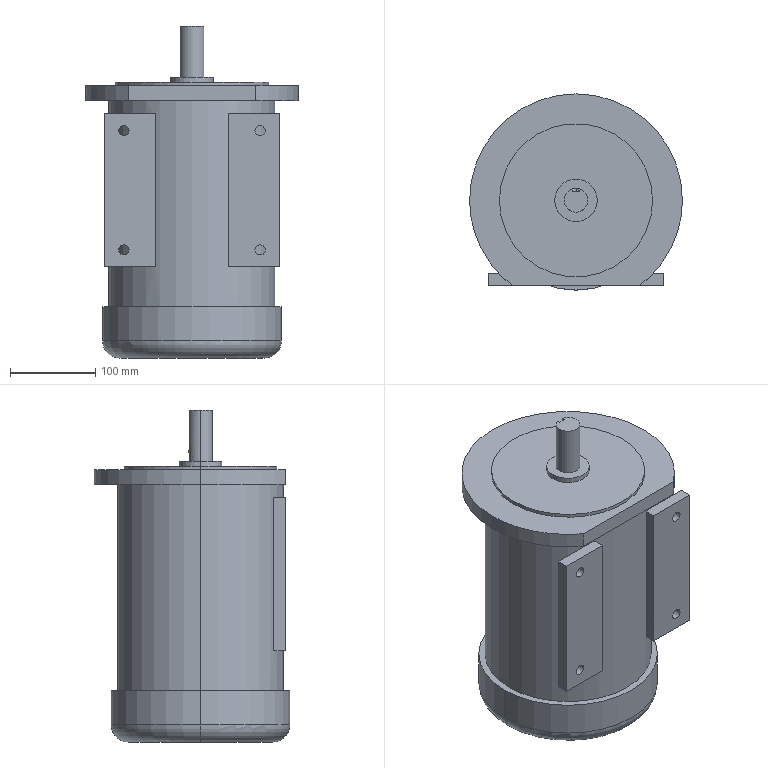Part | STEP file | Produce dryer line heating fan-MOYOT-Y100L2-4(3KW) | 1 solid | 48 faces | box 250 x 230 x 390 mm | volume 10532784 mm3 | cylinder 23 | plane 23 | torus 2 | commonest cylinder face diameters 12 x8 250 x3 8 x2 28 x2 50 x2 180 x2
STEP:
#1=CARTESIAN_POINT('',(74.,-100.,-193.));
#2=VERTEX_POINT('',#1);
#3=CARTESIAN_POINT('',(86.,-100.,-193.));
#4=VERTEX_POINT('',#3);
#5=CARTESIAN_POINT('',(80.,-100.,-193.));
#6=DIRECTION('',(0.,-1.,0.));
#7=DIRECTION('',(1.,0.,0.));
#8=AXIS2_PLACEMENT_3D('',#5,#6,#7);
#9=CIRCLE('',#8,6.);
#10=EDGE_CURVE('',#2,#4,#9,.T.);
#11=ORIENTED_EDGE('',*,*,#10,.T.);
#12=CARTESIAN_POINT('',(86.,-86.,-193.));
#13=VERTEX_POINT('',#12);
#14=CARTESIAN_POINT('',(86.,-100.,-193.));
#15=DIRECTION('',(0.,1.,0.));
#16=VECTOR('',#15,1000.);
#17=LINE('',#14,#16);
#18=EDGE_CURVE('',#4,#13,#17,.T.);
#19=ORIENTED_EDGE('',*,*,#18,.T.);
#20=CARTESIAN_POINT('',(74.,-86.,-193.));
#21=VERTEX_POINT('',#20);
#22=CARTESIAN_POINT('',(80.,-86.,-193.));
#23=DIRECTION('',(0.,-1.,0.));
#24=DIRECTION('',(1.,0.,0.));
#25=AXIS2_PLACEMENT_3D('',#22,#23,#24);
#26=CIRCLE('',#25,6.);
#27=EDGE_CURVE('',#21,#13,#26,.T.);
#28=ORIENTED_EDGE('',*,*,#27,.F.);
#29=CARTESIAN_POINT('',(74.,-100.,-193.));
#30=DIRECTION('',(0.,1.,0.));
#31=VECTOR('',#30,1000.);
#32=LINE('',#29,#31);
#33=EDGE_CURVE('',#2,#21,#32,.T.);
#34=ORIENTED_EDGE('',*,*,#33,.F.);
#35=EDGE_LOOP('',(#11,#19,#28,#34));
#36=FACE_OUTER_BOUND('',#35,.T.);
#37=CARTESIAN_POINT('',(80.,-100.,-193.));
#38=DIRECTION('',(0.,1.,0.));
#39=DIRECTION('',(-1.,0.,0.));
#40=AXIS2_PLACEMENT_3D('',#37,#38,#39);
#41=CYLINDRICAL_SURFACE('',#40,6.);
#42=ADVANCED_FACE('',(#36),#41,.F.);
#43=CARTESIAN_POINT('',(74.,-100.,-53.));
#44=VERTEX_POINT('',#43);
#45=CARTESIAN_POINT('',(86.,-100.,-53.));
#46=VERTEX_POINT('',#45);
#47=CARTESIAN_POINT('',(80.,-100.,-53.));
#48=DIRECTION('',(0.,-1.,0.));
#49=DIRECTION('',(1.,0.,0.));
#50=AXIS2_PLACEMENT_3D('',#47,#48,#49);
#51=CIRCLE('',#50,6.);
#52=EDGE_CURVE('',#44,#46,#51,.T.);
#53=ORIENTED_EDGE('',*,*,#52,.T.);
#54=CARTESIAN_POINT('',(86.,-86.,-53.));
#55=VERTEX_POINT('',#54);
#56=CARTESIAN_POINT('',(86.,-100.,-53.));
#57=DIRECTION('',(0.,1.,0.));
#58=VECTOR('',#57,1000.);
#59=LINE('',#56,#58);
#60=EDGE_CURVE('',#46,#55,#59,.T.);
#61=ORIENTED_EDGE('',*,*,#60,.T.);
#62=CARTESIAN_POINT('',(74.,-86.,-53.));
#63=VERTEX_POINT('',#62);
#64=CARTESIAN_POINT('',(80.,-86.,-53.));
#65=DIRECTION('',(0.,-1.,0.));
#66=DIRECTION('',(1.,0.,0.));
#67=AXIS2_PLACEMENT_3D('',#64,#65,#66);
#68=CIRCLE('',#67,6.);
#69=EDGE_CURVE('',#63,#55,#68,.T.);
#70=ORIENTED_EDGE('',*,*,#69,.F.);
#71=CARTESIAN_POINT('',(74.,-100.,-53.));
#72=DIRECTION('',(0.,1.,0.));
#73=VECTOR('',#72,1000.);
#74=LINE('',#71,#73);
#75=EDGE_CURVE('',#44,#63,#74,.T.);
#76=ORIENTED_EDGE('',*,*,#75,.F.);
#77=EDGE_LOOP('',(#53,#61,#70,#76));
#78=FACE_OUTER_BOUND('',#77,.T.);
#79=CARTESIAN_POINT('',(80.,-100.,-53.));
#80=DIRECTION('',(0.,1.,0.));
#81=DIRECTION('',(-1.,0.,0.));
#82=AXIS2_PLACEMENT_3D('',#79,#80,#81);
#83=CYLINDRICAL_SURFACE('',#82,6.);
#84=ADVANCED_FACE('',(#78),#83,.F.);
#85=CARTESIAN_POINT('',(-74.,-100.,-193.));
#86=VERTEX_POINT('',#85);
#87=CARTESIAN_POINT('',(-86.,-100.,-193.));
#88=VERTEX_POINT('',#87);
#89=CARTESIAN_POINT('',(-80.,-100.,-193.));
#90=DIRECTION('',(0.,1.,0.));
#91=DIRECTION('',(-1.,0.,0.));
#92=AXIS2_PLACEMENT_3D('',#89,#90,#91);
#93=CIRCLE('',#92,6.);
#94=EDGE_CURVE('',#86,#88,#93,.T.);
#95=ORIENTED_EDGE('',*,*,#94,.F.);
#96=CARTESIAN_POINT('',(-74.,-86.,-193.));
#97=VERTEX_POINT('',#96);
#98=CARTESIAN_POINT('',(-74.,-100.,-193.));
#99=DIRECTION('',(0.,1.,0.));
#100=VECTOR('',#99,1000.);
#101=LINE('',#98,#100);
#102=EDGE_CURVE('',#86,#97,#101,.T.);
#103=ORIENTED_EDGE('',*,*,#102,.T.);
#104=CARTESIAN_POINT('',(-86.,-86.,-193.));
#105=VERTEX_POINT('',#104);
#106=CARTESIAN_POINT('',(-80.,-86.,-193.));
#107=DIRECTION('',(0.,1.,0.));
#108=DIRECTION('',(-1.,0.,0.));
#109=AXIS2_PLACEMENT_3D('',#106,#107,#108);
#110=CIRCLE('',#109,6.);
#111=EDGE_CURVE('',#97,#105,#110,.T.);
#112=ORIENTED_EDGE('',*,*,#111,.T.);
#113=CARTESIAN_POINT('',(-86.,-100.,-193.));
#114=DIRECTION('',(0.,1.,0.));
#115=VECTOR('',#114,1000.);
#116=LINE('',#113,#115);
#117=EDGE_CURVE('',#88,#105,#116,.T.);
#118=ORIENTED_EDGE('',*,*,#117,.F.);
#119=EDGE_LOOP('',(#95,#103,#112,#118));
#120=FACE_OUTER_BOUND('',#119,.T.);
#121=CARTESIAN_POINT('',(-80.,-100.,-193.));
#122=DIRECTION('',(0.,1.,0.));
#123=DIRECTION('',(-1.,0.,0.));
#124=AXIS2_PLACEMENT_3D('',#121,#122,#123);
#125=CYLINDRICAL_SURFACE('',#124,6.);
#126=ADVANCED_FACE('',(#120),#125,.F.);
#127=CARTESIAN_POINT('',(-74.,-100.,-53.));
#128=VERTEX_POINT('',#127);
#129=CARTESIAN_POINT('',(-86.,-100.,-53.));
#130=VERTEX_POINT('',#129);
#131=CARTESIAN_POINT('',(-80.,-100.,-53.));
#132=DIRECTION('',(0.,1.,0.));
#133=DIRECTION('',(-1.,0.,0.));
#134=AXIS2_PLACEMENT_3D('',#131,#132,#133);
#135=CIRCLE('',#134,6.);
#136=EDGE_CURVE('',#128,#130,#135,.T.);
#137=ORIENTED_EDGE('',*,*,#136,.F.);
#138=CARTESIAN_POINT('',(-74.,-86.,-53.));
#139=VERTEX_POINT('',#138);
#140=CARTESIAN_POINT('',(-74.,-100.,-53.));
#141=DIRECTION('',(0.,1.,0.));
#142=VECTOR('',#141,1000.);
#143=LINE('',#140,#142);
#144=EDGE_CURVE('',#128,#139,#143,.T.);
#145=ORIENTED_EDGE('',*,*,#144,.T.);
#146=CARTESIAN_POINT('',(-86.,-86.,-53.));
#147=VERTEX_POINT('',#146);
#148=CARTESIAN_POINT('',(-80.,-86.,-53.));
#149=DIRECTION('',(0.,1.,0.));
#150=DIRECTION('',(-1.,0.,0.));
#151=AXIS2_PLACEMENT_3D('',#148,#149,#150);
#152=CIRCLE('',#151,6.);
#153=EDGE_CURVE('',#139,#147,#152,.T.);
#154=ORIENTED_EDGE('',*,*,#153,.T.);
#155=CARTESIAN_POINT('',(-86.,-100.,-53.));
#156=DIRECTION('',(0.,1.,0.));
#157=VECTOR('',#156,1000.);
#158=LINE('',#155,#157);
#159=EDGE_CURVE('',#130,#147,#158,.T.);
#160=ORIENTED_EDGE('',*,*,#159,.F.);
#161=EDGE_LOOP('',(#137,#145,#154,#160));
#162=FACE_OUTER_BOUND('',#161,.T.);
#163=CARTESIAN_POINT('',(-80.,-100.,-53.));
#164=DIRECTION('',(0.,1.,0.));
#165=DIRECTION('',(-1.,0.,0.));
#166=AXIS2_PLACEMENT_3D('',#163,#164,#165);
#167=CYLINDRICAL_SURFACE('',#166,6.);
#168=ADVANCED_FACE('',(#162),#167,.F.);
#169=CARTESIAN_POINT('',(105.,0.,-300.));
#170=VERTEX_POINT('',#169);
#171=CARTESIAN_POINT('',(-105.,0.,-300.));
#172=VERTEX_POINT('',#171);
#173=CARTESIAN_POINT('',(0.,0.,-300.));
#174=DIRECTION('',(0.,0.,1.));
#175=DIRECTION('',(-1.,0.,0.));
#176=AXIS2_PLACEMENT_3D('',#173,#174,#175);
#177=CIRCLE('',#176,105.);
#178=EDGE_CURVE('',#170,#172,#177,.T.);
#179=ORIENTED_EDGE('',*,*,#178,.F.);
#180=CARTESIAN_POINT('',(85.,0.,-320.));
#181=VERTEX_POINT('',#180);
#182=CARTESIAN_POINT('',(85.,0.,-300.));
#183=DIRECTION('',(0.,1.,0.));
#184=DIRECTION('',(-1.,0.,0.));
#185=AXIS2_PLACEMENT_3D('',#182,#183,#184);
#186=CIRCLE('',#185,20.);
#187=EDGE_CURVE('',#170,#181,#186,.T.);
#188=ORIENTED_EDGE('',*,*,#187,.T.);
#189=CARTESIAN_POINT('',(-85.,0.,-320.));
#190=VERTEX_POINT('',#189);
#191=CARTESIAN_POINT('',(0.,0.,-320.));
#192=DIRECTION('',(0.,0.,-1.));
#193=DIRECTION('',(-1.,0.,0.));
#194=AXIS2_PLACEMENT_3D('',#191,#192,#193);
#195=CIRCLE('',#194,85.);
#196=EDGE_CURVE('',#190,#181,#195,.T.);
#197=ORIENTED_EDGE('',*,*,#196,.F.);
#198=CARTESIAN_POINT('',(-85.,0.,-300.));
#199=DIRECTION('',(0.,-1.,0.));
#200=DIRECTION('',(0.,0.,-1.));
#201=AXIS2_PLACEMENT_3D('',#198,#199,#200);
#202=CIRCLE('',#201,20.);
#203=EDGE_CURVE('',#172,#190,#202,.T.);
#204=ORIENTED_EDGE('',*,*,#203,.F.);
#205=EDGE_LOOP('',(#179,#188,#197,#204));
#206=FACE_OUTER_BOUND('',#205,.T.);
#207=CARTESIAN_POINT('',(0.,0.,-300.));
#208=DIRECTION('',(0.,0.,-1.));
#209=DIRECTION('',(-1.,0.,0.));
#210=AXIS2_PLACEMENT_3D('',#207,#208,#209);
#211=TOROIDAL_SURFACE('',#210,85.,20.);
#212=ADVANCED_FACE('',(#206),#211,.T.);
#213=ORIENTED_EDGE('',*,*,#178,.T.);
#214=CARTESIAN_POINT('',(-105.,0.,-260.));
#215=VERTEX_POINT('',#214);
#216=CARTESIAN_POINT('',(-105.,0.,-320.));
#217=DIRECTION('',(0.,0.,1.));
#218=VECTOR('',#217,1000.);
#219=LINE('',#216,#218);
#220=EDGE_CURVE('',#172,#215,#219,.T.);
#221=ORIENTED_EDGE('',*,*,#220,.T.);
#222=CARTESIAN_POINT('',(105.,0.,-260.));
#223=VERTEX_POINT('',#222);
#224=CARTESIAN_POINT('',(0.,0.,-260.));
#225=DIRECTION('',(0.,0.,-1.));
#226=DIRECTION('',(-1.,0.,0.));
#227=AXIS2_PLACEMENT_3D('',#224,#225,#226);
#228=CIRCLE('',#227,105.);
#229=EDGE_CURVE('',#215,#223,#228,.T.);
#230=ORIENTED_EDGE('',*,*,#229,.T.);
#231=CARTESIAN_POINT('',(105.,0.,-320.));
#232=DIRECTION('',(0.,0.,1.));
#233=VECTOR('',#232,1000.);
#234=LINE('',#231,#233);
#235=EDGE_CURVE('',#170,#223,#234,.T.);
#236=ORIENTED_EDGE('',*,*,#235,.F.);
#237=EDGE_LOOP('',(#213,#221,#230,#236));
#238=FACE_OUTER_BOUND('',#237,.T.);
#239=CARTESIAN_POINT('',(0.,0.,-320.));
#240=DIRECTION('',(0.,0.,1.));
#241=DIRECTION('',(1.,0.,0.));
#242=AXIS2_PLACEMENT_3D('',#239,#240,#241);
#243=CYLINDRICAL_SURFACE('',#242,105.);
#244=ADVANCED_FACE('',(#238),#243,.T.);
#245=CARTESIAN_POINT('',(-97.5,0.,-260.));
#246=VERTEX_POINT('',#245);
#247=CARTESIAN_POINT('',(97.5,0.,-260.));
#248=VERTEX_POINT('',#247);
#249=CARTESIAN_POINT('',(0.,0.,-260.));
#250=DIRECTION('',(0.,0.,-1.));
#251=DIRECTION('',(-1.,0.,0.));
#252=AXIS2_PLACEMENT_3D('',#249,#250,#251);
#253=CIRCLE('',#252,97.5);
#254=EDGE_CURVE('',#246,#248,#253,.T.);
#255=ORIENTED_EDGE('',*,*,#254,.F.);
#256=CARTESIAN_POINT('',(-97.5,0.,-18.));
#257=VERTEX_POINT('',#256);
#258=CARTESIAN_POINT('',(-97.5,0.,-260.));
#259=DIRECTION('',(0.,0.,1.));
#260=VECTOR('',#259,1000.);
#261=LINE('',#258,#260);
#262=EDGE_CURVE('',#246,#257,#261,.T.);
#263=ORIENTED_EDGE('',*,*,#262,.T.);
#264=CARTESIAN_POINT('',(97.5,0.,-18.));
#265=VERTEX_POINT('',#264);
#266=CARTESIAN_POINT('',(0.,0.,-18.));
#267=DIRECTION('',(0.,0.,-1.));
#268=DIRECTION('',(1.,0.,0.));
#269=AXIS2_PLACEMENT_3D('',#266,#267,#268);
#270=CIRCLE('',#269,97.5);
#271=EDGE_CURVE('',#257,#265,#270,.T.);
#272=ORIENTED_EDGE('',*,*,#271,.T.);
#273=CARTESIAN_POINT('',(97.5,0.,-260.));
#274=DIRECTION('',(0.,0.,1.));
#275=VECTOR('',#274,1000.);
#276=LINE('',#273,#275);
#277=EDGE_CURVE('',#248,#265,#276,.T.);
#278=ORIENTED_EDGE('',*,*,#277,.F.);
#279=EDGE_LOOP('',(#255,#263,#272,#278));
#280=FACE_OUTER_BOUND('',#279,.T.);
#281=CARTESIAN_POINT('',(0.,0.,-260.));
#282=DIRECTION('',(0.,0.,1.));
#283=DIRECTION('',(1.,0.,0.));
#284=AXIS2_PLACEMENT_3D('',#281,#282,#283);
#285=CYLINDRICAL_SURFACE('',#284,97.5);
#286=ADVANCED_FACE('',(#280),#285,.T.);
#287=CARTESIAN_POINT('',(14.,0.,70.));
#288=VERTEX_POINT('',#287);
#289=CARTESIAN_POINT('',(4.,13.416,70.));
#290=VERTEX_POINT('',#289);
#291=CARTESIAN_POINT('',(0.,0.,70.));
#292=DIRECTION('',(0.,0.,1.));
#293=DIRECTION('',(1.,0.,0.));
#294=AXIS2_PLACEMENT_3D('',#291,#292,#293);
#295=CIRCLE('',#294,14.);
#296=EDGE_CURVE('',#288,#290,#295,.T.);
#297=ORIENTED_EDGE('',*,*,#296,.F.);
#298=CARTESIAN_POINT('',(14.,0.,10.));
#299=VERTEX_POINT('',#298);
#300=CARTESIAN_POINT('',(14.,0.,70.));
#301=DIRECTION('',(0.,0.,-1.));
#302=VECTOR('',#301,1000.);
#303=LINE('',#300,#302);
#304=EDGE_CURVE('',#288,#299,#303,.T.);
#305=ORIENTED_EDGE('',*,*,#304,.T.);
#306=CARTESIAN_POINT('',(-14.,0.,10.));
#307=VERTEX_POINT('',#306);
#308=CARTESIAN_POINT('',(0.,0.,10.));
#309=DIRECTION('',(0.,0.,1.));
#310=DIRECTION('',(1.,0.,0.));
#311=AXIS2_PLACEMENT_3D('',#308,#309,#310);
#312=CIRCLE('',#311,14.);
#313=EDGE_CURVE('',#299,#307,#312,.T.);
#314=ORIENTED_EDGE('',*,*,#313,.T.);
#315=CARTESIAN_POINT('',(-14.,0.,70.));
#316=VERTEX_POINT('',#315);
#317=CARTESIAN_POINT('',(-14.,0.,70.));
#318=DIRECTION('',(0.,0.,-1.));
#319=VECTOR('',#318,1000.);
#320=LINE('',#317,#319);
#321=EDGE_CURVE('',#316,#307,#320,.T.);
#322=ORIENTED_EDGE('',*,*,#321,.F.);
#323=CARTESIAN_POINT('',(-4.,13.416,70.));
#324=VERTEX_POINT('',#323);
#325=CARTESIAN_POINT('',(0.,0.,70.));
#326=DIRECTION('',(0.,0.,1.));
#327=DIRECTION('',(1.,0.,0.));
#328=AXIS2_PLACEMENT_3D('',#325,#326,#327);
#329=CIRCLE('',#328,14.);
#330=EDGE_CURVE('',#324,#316,#329,.T.);
#331=ORIENTED_EDGE('',*,*,#330,.F.);
#332=CARTESIAN_POINT('',(-4.,13.416,24.));
#333=VERTEX_POINT('',#332);
#334=CARTESIAN_POINT('',(-4.,13.416,70.));
#335=DIRECTION('',(0.,0.,-1.));
#336=VECTOR('',#335,1000.);
#337=LINE('',#334,#336);
#338=EDGE_CURVE('',#324,#333,#337,.T.);
#339=ORIENTED_EDGE('',*,*,#338,.T.);
#340=CARTESIAN_POINT('',(0.,14.,20.));
#341=VERTEX_POINT('',#340);
#342=CARTESIAN_POINT('',(-4.,13.416,24.));
#343=CARTESIAN_POINT('',(-4.,13.416,23.734));
#344=CARTESIAN_POINT('',(-3.974,13.424,23.474));
#345=CARTESIAN_POINT('',(-3.871,13.454,22.961));
#346=CARTESIAN_POINT('',(-3.794,13.477,22.706));
#347=CARTESIAN_POINT('',(-3.593,13.531,22.223));
#348=CARTESIAN_POINT('',(-3.47,13.564,21.994));
#349=CARTESIAN_POINT('',(-3.18,13.635,21.56));
#350=CARTESIAN_POINT('',(-3.013,13.673,21.356));
#351=CARTESIAN_POINT('',(-2.646,13.749,20.989));
#352=CARTESIAN_POINT('',(-2.446,13.786,20.824));
#353=CARTESIAN_POINT('',(-2.009,13.857,20.531));
#354=CARTESIAN_POINT('',(-1.779,13.889,20.408));
#355=CARTESIAN_POINT('',(-1.299,13.942,20.208));
#356=CARTESIAN_POINT('',(-1.046,13.963,20.13));
#357=CARTESIAN_POINT('',(-0.5278,13.992,20.026));
#358=CARTESIAN_POINT('',(-0.2656,14.,20.));
#359=CARTESIAN_POINT('',(0.,14.,20.));
#360=B_SPLINE_CURVE_WITH_KNOTS('',3,(#342,#343,#344,#345,#346,#347,#348,#349,#350,#351,#352,#353,#354,#355,#356,#357,#358,#359),.UNSPECIFIED.,.F.,.F.,(4,2,2,2,2,2,2,2,4),(0.,0.0007852,0.00157,0.002356,0.003141,0.003926,0.004711,0.005496,0.006282),.UNSPECIFIED.);
#361=EDGE_CURVE('',#333,#341,#360,.T.);
#362=ORIENTED_EDGE('',*,*,#361,.T.);
#363=CARTESIAN_POINT('',(4.,13.416,24.));
#364=VERTEX_POINT('',#363);
#365=CARTESIAN_POINT('',(0.,14.,20.));
#366=CARTESIAN_POINT('',(0.2656,14.,20.));
#367=CARTESIAN_POINT('',(0.5265,13.992,20.026));
#368=CARTESIAN_POINT('',(1.039,13.964,20.129));
#369=CARTESIAN_POINT('',(1.294,13.942,20.206));
#370=CARTESIAN_POINT('',(1.778,13.889,20.407));
#371=CARTESIAN_POINT('',(2.007,13.857,20.53));
#372=CARTESIAN_POINT('',(2.44,13.787,20.82));
#373=CARTESIAN_POINT('',(2.645,13.749,20.988));
#374=CARTESIAN_POINT('',(3.011,13.674,21.354));
#375=CARTESIAN_POINT('',(3.176,13.636,21.555));
#376=CARTESIAN_POINT('',(3.469,13.564,21.991));
#377=CARTESIAN_POINT('',(3.592,13.532,22.221));
#378=CARTESIAN_POINT('',(3.792,13.477,22.702));
#379=CARTESIAN_POINT('',(3.87,13.455,22.954));
#380=CARTESIAN_POINT('',(3.974,13.424,23.472));
#381=CARTESIAN_POINT('',(4.,13.416,23.734));
#382=CARTESIAN_POINT('',(4.,13.416,24.));
#383=B_SPLINE_CURVE_WITH_KNOTS('',3,(#365,#366,#367,#368,#369,#370,#371,#372,#373,#374,#375,#376,#377,#378,#379,#380,#381,#382),.UNSPECIFIED.,.F.,.F.,(4,2,2,2,2,2,2,2,4),(0.,0.0007852,0.00157,0.002356,0.003141,0.003926,0.004711,0.005496,0.006282),.UNSPECIFIED.);
#384=EDGE_CURVE('',#341,#364,#383,.T.);
#385=ORIENTED_EDGE('',*,*,#384,.T.);
#386=CARTESIAN_POINT('',(4.,13.416,70.));
#387=DIRECTION('',(0.,0.,1.));
#388=VECTOR('',#387,1000.);
#389=LINE('',#386,#388);
#390=EDGE_CURVE('',#364,#290,#389,.T.);
#391=ORIENTED_EDGE('',*,*,#390,.T.);
#392=EDGE_LOOP('',(#297,#305,#314,#322,#331,#339,#362,#385,#391));
#393=FACE_OUTER_BOUND('',#392,.T.);
#394=CARTESIAN_POINT('',(0.,0.,70.));
#395=DIRECTION('',(0.,0.,-1.));
#396=DIRECTION('',(-1.,0.,0.));
#397=AXIS2_PLACEMENT_3D('',#394,#395,#396);
#398=CYLINDRICAL_SURFACE('',#397,14.);
#399=ADVANCED_FACE('',(#393),#398,.T.);
#400=CARTESIAN_POINT('',(25.,0.,10.));
#401=VERTEX_POINT('',#400);
#402=CARTESIAN_POINT('',(-25.,0.,10.));
#403=VERTEX_POINT('',#402);
#404=CARTESIAN_POINT('',(0.,0.,10.));
#405=DIRECTION('',(0.,0.,1.));
#406=DIRECTION('',(1.,0.,0.));
#407=AXIS2_PLACEMENT_3D('',#404,#405,#406);
#408=CIRCLE('',#407,25.);
#409=EDGE_CURVE('',#401,#403,#408,.T.);
#410=ORIENTED_EDGE('',*,*,#409,.F.);
#411=CARTESIAN_POINT('',(25.,0.,4.));
#412=VERTEX_POINT('',#411);
#413=CARTESIAN_POINT('',(25.,0.,10.));
#414=DIRECTION('',(0.,0.,-1.));
#415=VECTOR('',#414,1000.);
#416=LINE('',#413,#415);
#417=EDGE_CURVE('',#401,#412,#416,.T.);
#418=ORIENTED_EDGE('',*,*,#417,.T.);
#419=CARTESIAN_POINT('',(-25.,0.,4.));
#420=VERTEX_POINT('',#419);
#421=CARTESIAN_POINT('',(0.,0.,4.));
#422=DIRECTION('',(0.,0.,1.));
#423=DIRECTION('',(1.,0.,0.));
#424=AXIS2_PLACEMENT_3D('',#421,#422,#423);
#425=CIRCLE('',#424,25.);
#426=EDGE_CURVE('',#412,#420,#425,.T.);
#427=ORIENTED_EDGE('',*,*,#426,.T.);
#428=CARTESIAN_POINT('',(-25.,0.,10.));
#429=DIRECTION('',(0.,0.,-1.));
#430=VECTOR('',#429,1000.);
#431=LINE('',#428,#430);
#432=EDGE_CURVE('',#403,#420,#431,.T.);
#433=ORIENTED_EDGE('',*,*,#432,.F.);
#434=EDGE_LOOP('',(#410,#418,#427,#433));
#435=FACE_OUTER_BOUND('',#434,.T.);
#436=CARTESIAN_POINT('',(0.,0.,10.));
#437=DIRECTION('',(0.,0.,-1.));
#438=DIRECTION('',(-1.,0.,0.));
#439=AXIS2_PLACEMENT_3D('',#436,#437,#438);
#440=CYLINDRICAL_SURFACE('',#439,25.);
#441=ADVANCED_FACE('',(#435),#440,.T.);
#442=CARTESIAN_POINT('',(90.,0.,4.));
#443=VERTEX_POINT('',#442);
#444=CARTESIAN_POINT('',(-90.,0.,4.));
#445=VERTEX_POINT('',#444);
#446=CARTESIAN_POINT('',(0.,0.,4.));
#447=DIRECTION('',(0.,0.,1.));
#448=DIRECTION('',(1.,0.,0.));
#449=AXIS2_PLACEMENT_3D('',#446,#447,#448);
#450=CIRCLE('',#449,90.);
#451=EDGE_CURVE('',#443,#445,#450,.T.);
#452=ORIENTED_EDGE('',*,*,#451,.F.);
#453=CARTESIAN_POINT('',(90.,0.,0.));
#454=VERTEX_POINT('',#453);
#455=CARTESIAN_POINT('',(90.,0.,4.));
#456=DIRECTION('',(0.,0.,-1.));
#457=VECTOR('',#456,1000.);
#458=LINE('',#455,#457);
#459=EDGE_CURVE('',#443,#454,#458,.T.);
#460=ORIENTED_EDGE('',*,*,#459,.T.);
#461=CARTESIAN_POINT('',(-90.,0.,0.));
#462=VERTEX_POINT('',#461);
#463=CARTESIAN_POINT('',(0.,0.,0.));
#464=DIRECTION('',(0.,0.,1.));
#465=DIRECTION('',(1.,0.,0.));
#466=AXIS2_PLACEMENT_3D('',#463,#464,#465);
#467=CIRCLE('',#466,90.);
#468=EDGE_CURVE('',#454,#462,#467,.T.);
#469=ORIENTED_EDGE('',*,*,#468,.T.);
#470=CARTESIAN_POINT('',(-90.,0.,4.));
#471=DIRECTION('',(0.,0.,-1.));
#472=VECTOR('',#471,1000.);
#473=LINE('',#470,#472);
#474=EDGE_CURVE('',#445,#462,#473,.T.);
#475=ORIENTED_EDGE('',*,*,#474,.F.);
#476=EDGE_LOOP('',(#452,#460,#469,#475));
#477=FACE_OUTER_BOUND('',#476,.T.);
#478=CARTESIAN_POINT('',(0.,0.,4.));
#479=DIRECTION('',(0.,0.,-1.));
#480=DIRECTION('',(-1.,0.,0.));
#481=AXIS2_PLACEMENT_3D('',#478,#479,#480);
#482=CYLINDRICAL_SURFACE('',#481,90.);
#483=ADVANCED_FACE('',(#477),#482,.T.);
#484=CARTESIAN_POINT('',(125.,0.,-18.));
#485=VERTEX_POINT('',#484);
#486=CARTESIAN_POINT('',(-125.,0.,-18.));
#487=VERTEX_POINT('',#486);
#488=CARTESIAN_POINT('',(0.,0.,-18.));
#489=DIRECTION('',(0.,0.,1.));
#490=DIRECTION('',(1.,0.,0.));
#491=AXIS2_PLACEMENT_3D('',#488,#489,#490);
#492=CIRCLE('',#491,125.);
#493=EDGE_CURVE('',#485,#487,#492,.T.);
#494=ORIENTED_EDGE('',*,*,#493,.T.);
#495=CARTESIAN_POINT('',(-125.,0.,0.));
#496=VERTEX_POINT('',#495);
#497=CARTESIAN_POINT('',(-125.,0.,-18.));
#498=DIRECTION('',(0.,0.,1.));
#499=VECTOR('',#498,1000.);
#500=LINE('',#497,#499);
#501=EDGE_CURVE('',#487,#496,#500,.T.);
#502=ORIENTED_EDGE('',*,*,#501,.T.);
#503=CARTESIAN_POINT('',(125.,0.,0.));
#504=VERTEX_POINT('',#503);
#505=CARTESIAN_POINT('',(0.,0.,0.));
#506=DIRECTION('',(0.,0.,1.));
#507=DIRECTION('',(1.,0.,0.));
#508=AXIS2_PLACEMENT_3D('',#505,#506,#507);
#509=CIRCLE('',#508,125.);
#510=EDGE_CURVE('',#504,#496,#509,.T.);
#511=ORIENTED_EDGE('',*,*,#510,.F.);
#512=CARTESIAN_POINT('',(125.,0.,-18.));
#513=DIRECTION('',(0.,0.,1.));
#514=VECTOR('',#513,1000.);
#515=LINE('',#512,#514);
#516=EDGE_CURVE('',#485,#504,#515,.T.);
#517=ORIENTED_EDGE('',*,*,#516,.F.);
#518=EDGE_LOOP('',(#494,#502,#511,#517));
#519=FACE_OUTER_BOUND('',#518,.T.);
#520=CARTESIAN_POINT('',(0.,0.,-18.));
#521=DIRECTION('',(0.,0.,1.));
#522=DIRECTION('',(1.,0.,0.));
#523=AXIS2_PLACEMENT_3D('',#520,#521,#522);
#524=CYLINDRICAL_SURFACE('',#523,125.);
#525=ADVANCED_FACE('',(#519),#524,.T.);
#526=CARTESIAN_POINT('',(75.,-100.,-18.));
#527=VERTEX_POINT('',#526);
#528=CARTESIAN_POINT('',(0.,0.,-18.));
#529=DIRECTION('',(0.,0.,1.));
#530=DIRECTION('',(1.,0.,0.));
#531=AXIS2_PLACEMENT_3D('',#528,#529,#530);
#532=CIRCLE('',#531,125.);
#533=EDGE_CURVE('',#527,#485,#532,.T.);
#534=ORIENTED_EDGE('',*,*,#533,.T.);
#535=ORIENTED_EDGE('',*,*,#516,.T.);
#536=CARTESIAN_POINT('',(75.,-100.,0.));
#537=VERTEX_POINT('',#536);
#538=CARTESIAN_POINT('',(0.,0.,0.));
#539=DIRECTION('',(0.,0.,1.));
#540=DIRECTION('',(1.,0.,0.));
#541=AXIS2_PLACEMENT_3D('',#538,#539,#540);
#542=CIRCLE('',#541,125.);
#543=EDGE_CURVE('',#537,#504,#542,.T.);
#544=ORIENTED_EDGE('',*,*,#543,.F.);
#545=CARTESIAN_POINT('',(75.,-100.,-18.));
#546=DIRECTION('',(0.,0.,1.));
#547=VECTOR('',#546,1000.);
#548=LINE('',#545,#547);
#549=EDGE_CURVE('',#527,#537,#548,.T.);
#550=ORIENTED_EDGE('',*,*,#549,.F.);
#551=EDGE_LOOP('',(#534,#535,#544,#550));
#552=FACE_OUTER_BOUND('',#551,.T.);
#553=CARTESIAN_POINT('',(0.,0.,-18.));
#554=DIRECTION('',(0.,0.,1.));
#555=DIRECTION('',(1.,0.,0.));
#556=AXIS2_PLACEMENT_3D('',#553,#554,#555);
#557=CYLINDRICAL_SURFACE('',#556,125.);
#558=ADVANCED_FACE('',(#552),#557,.T.);
#559=ORIENTED_EDGE('',*,*,#69,.T.);
#560=CARTESIAN_POINT('',(80.,-86.,-53.));
#561=DIRECTION('',(0.,-1.,0.));
#562=DIRECTION('',(1.,0.,0.));
#563=AXIS2_PLACEMENT_3D('',#560,#561,#562);
#564=CIRCLE('',#563,6.);
#565=EDGE_CURVE('',#55,#63,#564,.T.);
#566=ORIENTED_EDGE('',*,*,#565,.T.);
#567=EDGE_LOOP('',(#559,#566));
#568=FACE_BOUND('',#567,.T.);
#569=CARTESIAN_POINT('',(45.937,-86.,-213.));
#570=VERTEX_POINT('',#569);
#571=CARTESIAN_POINT('',(102.5,-86.,-213.));
#572=VERTEX_POINT('',#571);
#573=CARTESIAN_POINT('',(102.5,-86.,-213.));
#574=DIRECTION('',(1.,0.,0.));
#575=VECTOR('',#574,1000.);
#576=LINE('',#573,#575);
#577=EDGE_CURVE('',#570,#572,#576,.T.);
#578=ORIENTED_EDGE('',*,*,#577,.F.);
#579=CARTESIAN_POINT('',(45.937,-86.,-33.));
#580=VERTEX_POINT('',#579);
#581=CARTESIAN_POINT('',(45.937,-86.,-260.));
#582=DIRECTION('',(0.,0.,1.));
#583=VECTOR('',#582,1000.);
#584=LINE('',#581,#583);
#585=EDGE_CURVE('',#570,#580,#584,.T.);
#586=ORIENTED_EDGE('',*,*,#585,.T.);
#587=CARTESIAN_POINT('',(102.5,-86.,-33.));
#588=VERTEX_POINT('',#587);
#589=CARTESIAN_POINT('',(102.5,-86.,-33.));
#590=DIRECTION('',(1.,0.,0.));
#591=VECTOR('',#590,1000.);
#592=LINE('',#589,#591);
#593=EDGE_CURVE('',#580,#588,#592,.T.);
#594=ORIENTED_EDGE('',*,*,#593,.T.);
#595=CARTESIAN_POINT('',(102.5,-86.,-213.));
#596=DIRECTION('',(0.,0.,1.));
#597=VECTOR('',#596,1000.);
#598=LINE('',#595,#597);
#599=EDGE_CURVE('',#572,#588,#598,.T.);
#600=ORIENTED_EDGE('',*,*,#599,.F.);
#601=EDGE_LOOP('',(#578,#586,#594,#600));
#602=FACE_OUTER_BOUND('',#601,.T.);
#603=ORIENTED_EDGE('',*,*,#27,.T.);
#604=CARTESIAN_POINT('',(80.,-86.,-193.));
#605=DIRECTION('',(0.,-1.,0.));
#606=DIRECTION('',(1.,0.,0.));
#607=AXIS2_PLACEMENT_3D('',#604,#605,#606);
#608=CIRCLE('',#607,6.);
#609=EDGE_CURVE('',#13,#21,#608,.T.);
#610=ORIENTED_EDGE('',*,*,#609,.T.);
#611=EDGE_LOOP('',(#603,#610));
#612=FACE_BOUND('',#611,.T.);
#613=CARTESIAN_POINT('',(102.5,-86.,-213.));
#614=DIRECTION('',(0.,-1.,0.));
#615=DIRECTION('',(0.,0.,-1.));
#616=AXIS2_PLACEMENT_3D('',#613,#614,#615);
#617=PLANE('',#616);
#618=ADVANCED_FACE('',(#568,#602,#612),#617,.F.);
#619=ORIENTED_EDGE('',*,*,#52,.F.);
#620=CARTESIAN_POINT('',(80.,-100.,-53.));
#621=DIRECTION('',(0.,-1.,0.));
#622=DIRECTION('',(1.,0.,0.));
#623=AXIS2_PLACEMENT_3D('',#620,#621,#622);
#624=CIRCLE('',#623,6.);
#625=EDGE_CURVE('',#46,#44,#624,.T.);
#626=ORIENTED_EDGE('',*,*,#625,.F.);
#627=EDGE_LOOP('',(#619,#626));
#628=FACE_BOUND('',#627,.T.);
#629=CARTESIAN_POINT('',(102.5,-100.,-33.));
#630=VERTEX_POINT('',#629);
#631=CARTESIAN_POINT('',(42.5,-100.,-33.));
#632=VERTEX_POINT('',#631);
#633=CARTESIAN_POINT('',(42.5,-100.,-33.));
#634=DIRECTION('',(-1.,0.,0.));
#635=VECTOR('',#634,1000.);
#636=LINE('',#633,#635);
#637=EDGE_CURVE('',#630,#632,#636,.T.);
#638=ORIENTED_EDGE('',*,*,#637,.T.);
#639=CARTESIAN_POINT('',(42.5,-100.,-213.));
#640=VERTEX_POINT('',#639);
#641=CARTESIAN_POINT('',(42.5,-100.,-213.));
#642=DIRECTION('',(0.,0.,1.));
#643=VECTOR('',#642,1000.);
#644=LINE('',#641,#643);
#645=EDGE_CURVE('',#640,#632,#644,.T.);
#646=ORIENTED_EDGE('',*,*,#645,.F.);
#647=CARTESIAN_POINT('',(102.5,-100.,-213.));
#648=VERTEX_POINT('',#647);
#649=CARTESIAN_POINT('',(42.5,-100.,-213.));
#650=DIRECTION('',(-1.,0.,0.));
#651=VECTOR('',#650,1000.);
#652=LINE('',#649,#651);
#653=EDGE_CURVE('',#648,#640,#652,.T.);
#654=ORIENTED_EDGE('',*,*,#653,.F.);
#655=CARTESIAN_POINT('',(102.5,-100.,-213.));
#656=DIRECTION('',(0.,0.,1.));
#657=VECTOR('',#656,1000.);
#658=LINE('',#655,#657);
#659=EDGE_CURVE('',#648,#630,#658,.T.);
#660=ORIENTED_EDGE('',*,*,#659,.T.);
#661=EDGE_LOOP('',(#638,#646,#654,#660));
#662=FACE_OUTER_BOUND('',#661,.T.);
#663=ORIENTED_EDGE('',*,*,#10,.F.);
#664=CARTESIAN_POINT('',(80.,-100.,-193.));
#665=DIRECTION('',(0.,-1.,0.));
#666=DIRECTION('',(1.,0.,0.));
#667=AXIS2_PLACEMENT_3D('',#664,#665,#666);
#668=CIRCLE('',#667,6.);
#669=EDGE_CURVE('',#4,#2,#668,.T.);
#670=ORIENTED_EDGE('',*,*,#669,.F.);
#671=EDGE_LOOP('',(#663,#670));
#672=FACE_BOUND('',#671,.T.);
#673=CARTESIAN_POINT('',(42.5,-100.,-213.));
#674=DIRECTION('',(0.,1.,0.));
#675=DIRECTION('',(0.,0.,1.));
#676=AXIS2_PLACEMENT_3D('',#673,#674,#675);
#677=PLANE('',#676);
#678=ADVANCED_FACE('',(#628,#662,#672),#677,.F.);
#679=ORIENTED_EDGE('',*,*,#533,.F.);
#680=CARTESIAN_POINT('',(-75.,-100.,-18.));
#681=VERTEX_POINT('',#680);
#682=CARTESIAN_POINT('',(0.,-100.,-18.));
#683=DIRECTION('',(-1.,0.,0.));
#684=VECTOR('',#683,1000.);
#685=LINE('',#682,#684);
#686=EDGE_CURVE('',#527,#681,#685,.T.);
#687=ORIENTED_EDGE('',*,*,#686,.T.);
#688=CARTESIAN_POINT('',(0.,0.,-18.));
#689=DIRECTION('',(0.,0.,1.));
#690=DIRECTION('',(1.,0.,0.));
#691=AXIS2_PLACEMENT_3D('',#688,#689,#690);
#692=CIRCLE('',#691,125.);
#693=EDGE_CURVE('',#487,#681,#692,.T.);
#694=ORIENTED_EDGE('',*,*,#693,.F.);
#695=ORIENTED_EDGE('',*,*,#493,.F.);
#696=EDGE_LOOP('',(#679,#687,#694,#695));
#697=FACE_OUTER_BOUND('',#696,.T.);
#698=CARTESIAN_POINT('',(0.,0.,-18.));
#699=DIRECTION('',(0.,0.,-1.));
#700=DIRECTION('',(1.,0.,0.));
#701=AXIS2_PLACEMENT_3D('',#698,#699,#700);
#702=CIRCLE('',#701,97.5);
#703=EDGE_CURVE('',#265,#257,#702,.T.);
#704=ORIENTED_EDGE('',*,*,#703,.F.);
#705=ORIENTED_EDGE('',*,*,#271,.F.);
#706=EDGE_LOOP('',(#704,#705));
#707=FACE_BOUND('',#706,.T.);
#708=CARTESIAN_POINT('',(0.,0.,-18.));
#709=DIRECTION('',(0.,0.,1.));
#710=DIRECTION('',(1.,0.,0.));
#711=AXIS2_PLACEMENT_3D('',#708,#709,#710);
#712=PLANE('',#711);
#713=ADVANCED_FACE('',(#697,#707),#712,.F.);
#714=CARTESIAN_POINT('',(0.,0.,10.));
#715=DIRECTION('',(0.,0.,1.));
#716=DIRECTION('',(1.,0.,0.));
#717=AXIS2_PLACEMENT_3D('',#714,#715,#716);
#718=CIRCLE('',#717,25.);
#719=EDGE_CURVE('',#403,#401,#718,.T.);
#720=ORIENTED_EDGE('',*,*,#719,.T.);
#721=ORIENTED_EDGE('',*,*,#409,.T.);
#722=EDGE_LOOP('',(#720,#721));
#723=FACE_OUTER_BOUND('',#722,.T.);
#724=CARTESIAN_POINT('',(0.,0.,10.));
#725=DIRECTION('',(0.,0.,1.));
#726=DIRECTION('',(1.,0.,0.));
#727=AXIS2_PLACEMENT_3D('',#724,#725,#726);
#728=CIRCLE('',#727,14.);
#729=EDGE_CURVE('',#307,#299,#728,.T.);
#730=ORIENTED_EDGE('',*,*,#729,.F.);
#731=ORIENTED_EDGE('',*,*,#313,.F.);
#732=EDGE_LOOP('',(#730,#731));
#733=FACE_BOUND('',#732,.T.);
#734=CARTESIAN_POINT('',(0.,0.,10.));
#735=DIRECTION('',(0.,0.,1.));
#736=DIRECTION('',(1.,0.,0.));
#737=AXIS2_PLACEMENT_3D('',#734,#735,#736);
#738=PLANE('',#737);
#739=ADVANCED_FACE('',(#723,#733),#738,.T.);
#740=CARTESIAN_POINT('',(0.,0.,4.));
#741=DIRECTION('',(0.,0.,1.));
#742=DIRECTION('',(1.,0.,0.));
#743=AXIS2_PLACEMENT_3D('',#740,#741,#742);
#744=CIRCLE('',#743,90.);
#745=EDGE_CURVE('',#445,#443,#744,.T.);
#746=ORIENTED_EDGE('',*,*,#745,.T.);
#747=ORIENTED_EDGE('',*,*,#451,.T.);
#748=EDGE_LOOP('',(#746,#747));
#749=FACE_OUTER_BOUND('',#748,.T.);
#750=CARTESIAN_POINT('',(0.,0.,4.));
#751=DIRECTION('',(0.,0.,1.));
#752=DIRECTION('',(1.,0.,0.));
#753=AXIS2_PLACEMENT_3D('',#750,#751,#752);
#754=CIRCLE('',#753,25.);
#755=EDGE_CURVE('',#420,#412,#754,.T.);
#756=ORIENTED_EDGE('',*,*,#755,.F.);
#757=ORIENTED_EDGE('',*,*,#426,.F.);
#758=EDGE_LOOP('',(#756,#757));
#759=FACE_BOUND('',#758,.T.);
#760=CARTESIAN_POINT('',(0.,0.,4.));
#761=DIRECTION('',(0.,0.,1.));
#762=DIRECTION('',(1.,0.,0.));
#763=AXIS2_PLACEMENT_3D('',#760,#761,#762);
#764=PLANE('',#763);
#765=ADVANCED_FACE('',(#749,#759),#764,.T.);
#766=CARTESIAN_POINT('',(-75.,-100.,0.));
#767=VERTEX_POINT('',#766);
#768=CARTESIAN_POINT('',(-85.268,-100.,0.));
#769=DIRECTION('',(-1.,0.,0.));
#770=VECTOR('',#769,1000.);
#771=LINE('',#768,#770);
#772=EDGE_CURVE('',#537,#767,#771,.T.);
#773=ORIENTED_EDGE('',*,*,#772,.F.);
#774=ORIENTED_EDGE('',*,*,#543,.T.);
#775=ORIENTED_EDGE('',*,*,#510,.T.);
#776=CARTESIAN_POINT('',(0.,0.,0.));
#777=DIRECTION('',(0.,0.,1.));
#778=DIRECTION('',(1.,0.,0.));
#779=AXIS2_PLACEMENT_3D('',#776,#777,#778);
#780=CIRCLE('',#779,125.);
#781=EDGE_CURVE('',#496,#767,#780,.T.);
#782=ORIENTED_EDGE('',*,*,#781,.T.);
#783=EDGE_LOOP('',(#773,#774,#775,#782));
#784=FACE_OUTER_BOUND('',#783,.T.);
#785=CARTESIAN_POINT('',(0.,0.,0.));
#786=DIRECTION('',(0.,0.,1.));
#787=DIRECTION('',(1.,0.,0.));
#788=AXIS2_PLACEMENT_3D('',#785,#786,#787);
#789=CIRCLE('',#788,90.);
#790=EDGE_CURVE('',#462,#454,#789,.T.);
#791=ORIENTED_EDGE('',*,*,#790,.F.);
#792=ORIENTED_EDGE('',*,*,#468,.F.);
#793=EDGE_LOOP('',(#791,#792));
#794=FACE_BOUND('',#793,.T.);
#795=CARTESIAN_POINT('',(0.,0.,0.));
#796=DIRECTION('',(0.,0.,1.));
#797=DIRECTION('',(1.,0.,0.));
#798=AXIS2_PLACEMENT_3D('',#795,#796,#797);
#799=PLANE('',#798);
#800=ADVANCED_FACE('',(#784,#794),#799,.T.);
#801=ORIENTED_EDGE('',*,*,#501,.F.);
#802=ORIENTED_EDGE('',*,*,#693,.T.);
#803=CARTESIAN_POINT('',(-75.,-100.,-18.));
#804=DIRECTION('',(0.,0.,-1.));
#805=VECTOR('',#804,1000.);
#806=LINE('',#803,#805);
#807=EDGE_CURVE('',#767,#681,#806,.T.);
#808=ORIENTED_EDGE('',*,*,#807,.F.);
#809=ORIENTED_EDGE('',*,*,#781,.F.);
#810=EDGE_LOOP('',(#801,#802,#808,#809));
#811=FACE_OUTER_BOUND('',#810,.T.);
#812=CARTESIAN_POINT('',(0.,0.,-18.));
#813=DIRECTION('',(0.,0.,1.));
#814=DIRECTION('',(1.,0.,0.));
#815=AXIS2_PLACEMENT_3D('',#812,#813,#814);
#816=CYLINDRICAL_SURFACE('',#815,125.);
#817=ADVANCED_FACE('',(#811),#816,.T.);
#818=ORIENTED_EDGE('',*,*,#459,.F.);
#819=ORIENTED_EDGE('',*,*,#745,.F.);
#820=ORIENTED_EDGE('',*,*,#474,.T.);
#821=ORIENTED_EDGE('',*,*,#790,.T.);
#822=EDGE_LOOP('',(#818,#819,#820,#821));
#823=FACE_OUTER_BOUND('',#822,.T.);
#824=CARTESIAN_POINT('',(0.,0.,4.));
#825=DIRECTION('',(0.,0.,-1.));
#826=DIRECTION('',(-1.,0.,0.));
#827=AXIS2_PLACEMENT_3D('',#824,#825,#826);
#828=CYLINDRICAL_SURFACE('',#827,90.);
#829=ADVANCED_FACE('',(#823),#828,.T.);
#830=ORIENTED_EDGE('',*,*,#417,.F.);
#831=ORIENTED_EDGE('',*,*,#719,.F.);
#832=ORIENTED_EDGE('',*,*,#432,.T.);
#833=ORIENTED_EDGE('',*,*,#755,.T.);
#834=EDGE_LOOP('',(#830,#831,#832,#833));
#835=FACE_OUTER_BOUND('',#834,.T.);
#836=CARTESIAN_POINT('',(0.,0.,10.));
#837=DIRECTION('',(0.,0.,-1.));
#838=DIRECTION('',(-1.,0.,0.));
#839=AXIS2_PLACEMENT_3D('',#836,#837,#838);
#840=CYLINDRICAL_SURFACE('',#839,25.);
#841=ADVANCED_FACE('',(#835),#840,.T.);
#842=ORIENTED_EDGE('',*,*,#304,.F.);
#843=CARTESIAN_POINT('',(0.,0.,70.));
#844=DIRECTION('',(0.,0.,1.));
#845=DIRECTION('',(1.,0.,0.));
#846=AXIS2_PLACEMENT_3D('',#843,#844,#845);
#847=CIRCLE('',#846,14.);
#848=EDGE_CURVE('',#316,#288,#847,.T.);
#849=ORIENTED_EDGE('',*,*,#848,.F.);
#850=ORIENTED_EDGE('',*,*,#321,.T.);
#851=ORIENTED_EDGE('',*,*,#729,.T.);
#852=EDGE_LOOP('',(#842,#849,#850,#851));
#853=FACE_OUTER_BOUND('',#852,.T.);
#854=CARTESIAN_POINT('',(0.,0.,70.));
#855=DIRECTION('',(0.,0.,-1.));
#856=DIRECTION('',(-1.,0.,0.));
#857=AXIS2_PLACEMENT_3D('',#854,#855,#856);
#858=CYLINDRICAL_SURFACE('',#857,14.);
#859=ADVANCED_FACE('',(#853),#858,.T.);
#860=CARTESIAN_POINT('',(-4.,10.,70.));
#861=VERTEX_POINT('',#860);
#862=CARTESIAN_POINT('',(-4.,0.,70.));
#863=DIRECTION('',(0.,-1.,0.));
#864=VECTOR('',#863,1000.);
#865=LINE('',#862,#864);
#866=EDGE_CURVE('',#324,#861,#865,.T.);
#867=ORIENTED_EDGE('',*,*,#866,.F.);
#868=ORIENTED_EDGE('',*,*,#330,.T.);
#869=ORIENTED_EDGE('',*,*,#848,.T.);
#870=ORIENTED_EDGE('',*,*,#296,.T.);
#871=CARTESIAN_POINT('',(4.,10.,70.));
#872=VERTEX_POINT('',#871);
#873=CARTESIAN_POINT('',(4.,18.,70.));
#874=DIRECTION('',(0.,1.,0.));
#875=VECTOR('',#874,1000.);
#876=LINE('',#873,#875);
#877=EDGE_CURVE('',#872,#290,#876,.T.);
#878=ORIENTED_EDGE('',*,*,#877,.F.);
#879=CARTESIAN_POINT('',(-4.,10.,70.));
#880=DIRECTION('',(1.,0.,0.));
#881=VECTOR('',#880,1000.);
#882=LINE('',#879,#881);
#883=EDGE_CURVE('',#861,#872,#882,.T.);
#884=ORIENTED_EDGE('',*,*,#883,.F.);
#885=EDGE_LOOP('',(#867,#868,#869,#870,#878,#884));
#886=FACE_OUTER_BOUND('',#885,.T.);
#887=CARTESIAN_POINT('',(0.,0.,70.));
#888=DIRECTION('',(0.,0.,1.));
#889=DIRECTION('',(1.,0.,0.));
#890=AXIS2_PLACEMENT_3D('',#887,#888,#889);
#891=PLANE('',#890);
#892=ADVANCED_FACE('',(#886),#891,.T.);
#893=ORIENTED_EDGE('',*,*,#262,.F.);
#894=CARTESIAN_POINT('',(0.,0.,-260.));
#895=DIRECTION('',(0.,0.,-1.));
#896=DIRECTION('',(-1.,0.,0.));
#897=AXIS2_PLACEMENT_3D('',#894,#895,#896);
#898=CIRCLE('',#897,97.5);
#899=EDGE_CURVE('',#248,#246,#898,.T.);
#900=ORIENTED_EDGE('',*,*,#899,.F.);
#901=ORIENTED_EDGE('',*,*,#277,.T.);
#902=ORIENTED_EDGE('',*,*,#703,.T.);
#903=EDGE_LOOP('',(#893,#900,#901,#902));
#904=FACE_OUTER_BOUND('',#903,.T.);
#905=ORIENTED_EDGE('',*,*,#585,.F.);
#906=CARTESIAN_POINT('',(42.5,-87.75,-213.));
#907=VERTEX_POINT('',#906);
#908=CARTESIAN_POINT('',(0.,0.,-213.));
#909=DIRECTION('',(0.,0.,-1.));
#910=DIRECTION('',(-1.,0.,0.));
#911=AXIS2_PLACEMENT_3D('',#908,#909,#910);
#912=CIRCLE('',#911,97.5);
#913=EDGE_CURVE('',#570,#907,#912,.T.);
#914=ORIENTED_EDGE('',*,*,#913,.T.);
#915=CARTESIAN_POINT('',(42.5,-87.75,-33.));
#916=VERTEX_POINT('',#915);
#917=CARTESIAN_POINT('',(42.5,-87.75,-260.));
#918=DIRECTION('',(0.,0.,-1.));
#919=VECTOR('',#918,1000.);
#920=LINE('',#917,#919);
#921=EDGE_CURVE('',#916,#907,#920,.T.);
#922=ORIENTED_EDGE('',*,*,#921,.F.);
#923=CARTESIAN_POINT('',(0.,0.,-33.));
#924=DIRECTION('',(0.,0.,-1.));
#925=DIRECTION('',(-1.,0.,0.));
#926=AXIS2_PLACEMENT_3D('',#923,#924,#925);
#927=CIRCLE('',#926,97.5);
#928=EDGE_CURVE('',#580,#916,#927,.T.);
#929=ORIENTED_EDGE('',*,*,#928,.F.);
#930=EDGE_LOOP('',(#905,#914,#922,#929));
#931=FACE_BOUND('',#930,.T.);
#932=CARTESIAN_POINT('',(-42.5,-87.75,-33.));
#933=VERTEX_POINT('',#932);
#934=CARTESIAN_POINT('',(-42.5,-87.75,-213.));
#935=VERTEX_POINT('',#934);
#936=CARTESIAN_POINT('',(-42.5,-87.75,-260.));
#937=DIRECTION('',(0.,0.,-1.));
#938=VECTOR('',#937,1000.);
#939=LINE('',#936,#938);
#940=EDGE_CURVE('',#933,#935,#939,.T.);
#941=ORIENTED_EDGE('',*,*,#940,.T.);
#942=CARTESIAN_POINT('',(-45.937,-86.,-213.));
#943=VERTEX_POINT('',#942);
#944=CARTESIAN_POINT('',(0.,0.,-213.));
#945=DIRECTION('',(0.,0.,-1.));
#946=DIRECTION('',(-1.,0.,0.));
#947=AXIS2_PLACEMENT_3D('',#944,#945,#946);
#948=CIRCLE('',#947,97.5);
#949=EDGE_CURVE('',#935,#943,#948,.T.);
#950=ORIENTED_EDGE('',*,*,#949,.T.);
#951=CARTESIAN_POINT('',(-45.937,-86.,-33.));
#952=VERTEX_POINT('',#951);
#953=CARTESIAN_POINT('',(-45.937,-86.,-260.));
#954=DIRECTION('',(0.,0.,1.));
#955=VECTOR('',#954,1000.);
#956=LINE('',#953,#955);
#957=EDGE_CURVE('',#943,#952,#956,.T.);
#958=ORIENTED_EDGE('',*,*,#957,.T.);
#959=CARTESIAN_POINT('',(0.,0.,-33.));
#960=DIRECTION('',(0.,0.,-1.));
#961=DIRECTION('',(-1.,0.,0.));
#962=AXIS2_PLACEMENT_3D('',#959,#960,#961);
#963=CIRCLE('',#962,97.5);
#964=EDGE_CURVE('',#933,#952,#963,.T.);
#965=ORIENTED_EDGE('',*,*,#964,.F.);
#966=EDGE_LOOP('',(#941,#950,#958,#965));
#967=FACE_BOUND('',#966,.T.);
#968=CARTESIAN_POINT('',(0.,0.,-260.));
#969=DIRECTION('',(0.,0.,1.));
#970=DIRECTION('',(1.,0.,0.));
#971=AXIS2_PLACEMENT_3D('',#968,#969,#970);
#972=CYLINDRICAL_SURFACE('',#971,97.5);
#973=ADVANCED_FACE('',(#904,#931,#967),#972,.T.);
#974=CARTESIAN_POINT('',(0.,0.,-260.));
#975=DIRECTION('',(0.,0.,-1.));
#976=DIRECTION('',(-1.,0.,0.));
#977=AXIS2_PLACEMENT_3D('',#974,#975,#976);
#978=CIRCLE('',#977,105.);
#979=EDGE_CURVE('',#223,#215,#978,.T.);
#980=ORIENTED_EDGE('',*,*,#979,.F.);
#981=ORIENTED_EDGE('',*,*,#229,.F.);
#982=EDGE_LOOP('',(#980,#981));
#983=FACE_OUTER_BOUND('',#982,.T.);
#984=ORIENTED_EDGE('',*,*,#899,.T.);
#985=ORIENTED_EDGE('',*,*,#254,.T.);
#986=EDGE_LOOP('',(#984,#985));
#987=FACE_BOUND('',#986,.T.);
#988=CARTESIAN_POINT('',(0.,0.,-260.));
#989=DIRECTION('',(0.,0.,-1.));
#990=DIRECTION('',(-1.,0.,0.));
#991=AXIS2_PLACEMENT_3D('',#988,#989,#990);
#992=PLANE('',#991);
#993=ADVANCED_FACE('',(#983,#987),#992,.F.);
#994=ORIENTED_EDGE('',*,*,#220,.F.);
#995=CARTESIAN_POINT('',(0.,0.,-300.));
#996=DIRECTION('',(0.,0.,1.));
#997=DIRECTION('',(-1.,0.,0.));
#998=AXIS2_PLACEMENT_3D('',#995,#996,#997);
#999=CIRCLE('',#998,105.);
#1000=EDGE_CURVE('',#172,#170,#999,.T.);
#1001=ORIENTED_EDGE('',*,*,#1000,.T.);
#1002=ORIENTED_EDGE('',*,*,#235,.T.);
#1003=ORIENTED_EDGE('',*,*,#979,.T.);
#1004=EDGE_LOOP('',(#994,#1001,#1002,#1003));
#1005=FACE_OUTER_BOUND('',#1004,.T.);
#1006=CARTESIAN_POINT('',(0.,0.,-320.));
#1007=DIRECTION('',(0.,0.,1.));
#1008=DIRECTION('',(1.,0.,0.));
#1009=AXIS2_PLACEMENT_3D('',#1006,#1007,#1008);
#1010=CYLINDRICAL_SURFACE('',#1009,105.);
#1011=ADVANCED_FACE('',(#1005),#1010,.T.);
#1012=ORIENTED_EDGE('',*,*,#196,.T.);
#1013=CARTESIAN_POINT('',(0.,0.,-320.));
#1014=DIRECTION('',(0.,0.,-1.));
#1015=DIRECTION('',(-1.,0.,0.));
#1016=AXIS2_PLACEMENT_3D('',#1013,#1014,#1015);
#1017=CIRCLE('',#1016,85.);
#1018=EDGE_CURVE('',#181,#190,#1017,.T.);
#1019=ORIENTED_EDGE('',*,*,#1018,.T.);
#1020=EDGE_LOOP('',(#1012,#1019));
#1021=FACE_OUTER_BOUND('',#1020,.T.);
#1022=CARTESIAN_POINT('',(0.,0.,-320.));
#1023=DIRECTION('',(0.,0.,-1.));
#1024=DIRECTION('',(-1.,0.,0.));
#1025=AXIS2_PLACEMENT_3D('',#1022,#1023,#1024);
#1026=PLANE('',#1025);
#1027=ADVANCED_FACE('',(#1021),#1026,.T.);
#1028=ORIENTED_EDGE('',*,*,#187,.F.);
#1029=ORIENTED_EDGE('',*,*,#1000,.F.);
#1030=ORIENTED_EDGE('',*,*,#203,.T.);
#1031=ORIENTED_EDGE('',*,*,#1018,.F.);
#1032=EDGE_LOOP('',(#1028,#1029,#1030,#1031));
#1033=FACE_OUTER_BOUND('',#1032,.T.);
#1034=CARTESIAN_POINT('',(0.,0.,-300.));
#1035=DIRECTION('',(0.,0.,-1.));
#1036=DIRECTION('',(-1.,0.,0.));
#1037=AXIS2_PLACEMENT_3D('',#1034,#1035,#1036);
#1038=TOROIDAL_SURFACE('',#1037,85.,20.);
#1039=ADVANCED_FACE('',(#1033),#1038,.T.);
#1040=ORIENTED_EDGE('',*,*,#940,.F.);
#1041=CARTESIAN_POINT('',(-42.5,-100.,-33.));
#1042=VERTEX_POINT('',#1041);
#1043=CARTESIAN_POINT('',(-42.5,-86.,-33.));
#1044=DIRECTION('',(0.,1.,0.));
#1045=VECTOR('',#1044,1000.);
#1046=LINE('',#1043,#1045);
#1047=EDGE_CURVE('',#1042,#933,#1046,.T.);
#1048=ORIENTED_EDGE('',*,*,#1047,.F.);
#1049=CARTESIAN_POINT('',(-42.5,-100.,-213.));
#1050=VERTEX_POINT('',#1049);
#1051=CARTESIAN_POINT('',(-42.5,-100.,-213.));
#1052=DIRECTION('',(0.,0.,1.));
#1053=VECTOR('',#1052,1000.);
#1054=LINE('',#1051,#1053);
#1055=EDGE_CURVE('',#1050,#1042,#1054,.T.);
#1056=ORIENTED_EDGE('',*,*,#1055,.F.);
#1057=CARTESIAN_POINT('',(-42.5,-86.,-213.));
#1058=DIRECTION('',(0.,1.,0.));
#1059=VECTOR('',#1058,1000.);
#1060=LINE('',#1057,#1059);
#1061=EDGE_CURVE('',#1050,#935,#1060,.T.);
#1062=ORIENTED_EDGE('',*,*,#1061,.T.);
#1063=EDGE_LOOP('',(#1040,#1048,#1056,#1062));
#1064=FACE_OUTER_BOUND('',#1063,.T.);
#1065=CARTESIAN_POINT('',(-42.5,-86.,-213.));
#1066=DIRECTION('',(1.,0.,0.));
#1067=DIRECTION('',(0.,0.,-1.));
#1068=AXIS2_PLACEMENT_3D('',#1065,#1066,#1067);
#1069=PLANE('',#1068);
#1070=ADVANCED_FACE('',(#1064),#1069,.T.);
#1071=CARTESIAN_POINT('',(-80.,-86.,-193.));
#1072=DIRECTION('',(0.,1.,0.));
#1073=DIRECTION('',(-1.,0.,0.));
#1074=AXIS2_PLACEMENT_3D('',#1071,#1072,#1073);
#1075=CIRCLE('',#1074,6.);
#1076=EDGE_CURVE('',#105,#97,#1075,.T.);
#1077=ORIENTED_EDGE('',*,*,#1076,.F.);
#1078=ORIENTED_EDGE('',*,*,#111,.F.);
#1079=EDGE_LOOP('',(#1077,#1078));
#1080=FACE_BOUND('',#1079,.T.);
#1081=CARTESIAN_POINT('',(-80.,-86.,-53.));
#1082=DIRECTION('',(0.,1.,0.));
#1083=DIRECTION('',(-1.,0.,0.));
#1084=AXIS2_PLACEMENT_3D('',#1081,#1082,#1083);
#1085=CIRCLE('',#1084,6.);
#1086=EDGE_CURVE('',#147,#139,#1085,.T.);
#1087=ORIENTED_EDGE('',*,*,#1086,.F.);
#1088=ORIENTED_EDGE('',*,*,#153,.F.);
#1089=EDGE_LOOP('',(#1087,#1088));
#1090=FACE_BOUND('',#1089,.T.);
#1091=ORIENTED_EDGE('',*,*,#957,.F.);
#1092=CARTESIAN_POINT('',(-102.5,-86.,-213.));
#1093=VERTEX_POINT('',#1092);
#1094=CARTESIAN_POINT('',(-102.5,-86.,-213.));
#1095=DIRECTION('',(-1.,0.,0.));
#1096=VECTOR('',#1095,1000.);
#1097=LINE('',#1094,#1096);
#1098=EDGE_CURVE('',#943,#1093,#1097,.T.);
#1099=ORIENTED_EDGE('',*,*,#1098,.T.);
#1100=CARTESIAN_POINT('',(-102.5,-86.,-33.));
#1101=VERTEX_POINT('',#1100);
#1102=CARTESIAN_POINT('',(-102.5,-86.,-213.));
#1103=DIRECTION('',(0.,0.,1.));
#1104=VECTOR('',#1103,1000.);
#1105=LINE('',#1102,#1104);
#1106=EDGE_CURVE('',#1093,#1101,#1105,.T.);
#1107=ORIENTED_EDGE('',*,*,#1106,.T.);
#1108=CARTESIAN_POINT('',(-102.5,-86.,-33.));
#1109=DIRECTION('',(-1.,0.,0.));
#1110=VECTOR('',#1109,1000.);
#1111=LINE('',#1108,#1110);
#1112=EDGE_CURVE('',#952,#1101,#1111,.T.);
#1113=ORIENTED_EDGE('',*,*,#1112,.F.);
#1114=EDGE_LOOP('',(#1091,#1099,#1107,#1113));
#1115=FACE_OUTER_BOUND('',#1114,.T.);
#1116=CARTESIAN_POINT('',(-102.5,-86.,-213.));
#1117=DIRECTION('',(0.,1.,0.));
#1118=DIRECTION('',(0.,0.,1.));
#1119=AXIS2_PLACEMENT_3D('',#1116,#1117,#1118);
#1120=PLANE('',#1119);
#1121=ADVANCED_FACE('',(#1080,#1090,#1115),#1120,.T.);
#1122=ORIENTED_EDGE('',*,*,#949,.F.);
#1123=ORIENTED_EDGE('',*,*,#1061,.F.);
#1124=CARTESIAN_POINT('',(-102.5,-100.,-213.));
#1125=VERTEX_POINT('',#1124);
#1126=CARTESIAN_POINT('',(-42.5,-100.,-213.));
#1127=DIRECTION('',(1.,0.,0.));
#1128=VECTOR('',#1127,1000.);
#1129=LINE('',#1126,#1128);
#1130=EDGE_CURVE('',#1125,#1050,#1129,.T.);
#1131=ORIENTED_EDGE('',*,*,#1130,.F.);
#1132=CARTESIAN_POINT('',(-102.5,-100.,-213.));
#1133=DIRECTION('',(0.,-1.,0.));
#1134=VECTOR('',#1133,1000.);
#1135=LINE('',#1132,#1134);
#1136=EDGE_CURVE('',#1093,#1125,#1135,.T.);
#1137=ORIENTED_EDGE('',*,*,#1136,.F.);
#1138=ORIENTED_EDGE('',*,*,#1098,.F.);
#1139=EDGE_LOOP('',(#1122,#1123,#1131,#1137,#1138));
#1140=FACE_OUTER_BOUND('',#1139,.T.);
#1141=CARTESIAN_POINT('',(-42.5,-100.,-213.));
#1142=DIRECTION('',(0.,0.,-1.));
#1143=DIRECTION('',(-1.,0.,0.));
#1144=AXIS2_PLACEMENT_3D('',#1141,#1142,#1143);
#1145=PLANE('',#1144);
#1146=ADVANCED_FACE('',(#1140),#1145,.T.);
#1147=ORIENTED_EDGE('',*,*,#1047,.T.);
#1148=ORIENTED_EDGE('',*,*,#964,.T.);
#1149=ORIENTED_EDGE('',*,*,#1112,.T.);
#1150=CARTESIAN_POINT('',(-102.5,-100.,-33.));
#1151=VERTEX_POINT('',#1150);
#1152=CARTESIAN_POINT('',(-102.5,-100.,-33.));
#1153=DIRECTION('',(0.,-1.,0.));
#1154=VECTOR('',#1153,1000.);
#1155=LINE('',#1152,#1154);
#1156=EDGE_CURVE('',#1101,#1151,#1155,.T.);
#1157=ORIENTED_EDGE('',*,*,#1156,.T.);
#1158=CARTESIAN_POINT('',(-42.5,-100.,-33.));
#1159=DIRECTION('',(1.,0.,0.));
#1160=VECTOR('',#1159,1000.);
#1161=LINE('',#1158,#1160);
#1162=EDGE_CURVE('',#1151,#1042,#1161,.T.);
#1163=ORIENTED_EDGE('',*,*,#1162,.T.);
#1164=EDGE_LOOP('',(#1147,#1148,#1149,#1157,#1163));
#1165=FACE_OUTER_BOUND('',#1164,.T.);
#1166=CARTESIAN_POINT('',(-42.5,-100.,-33.));
#1167=DIRECTION('',(0.,0.,-1.));
#1168=DIRECTION('',(-1.,0.,0.));
#1169=AXIS2_PLACEMENT_3D('',#1166,#1167,#1168);
#1170=PLANE('',#1169);
#1171=ADVANCED_FACE('',(#1165),#1170,.F.);
#1172=CARTESIAN_POINT('',(-80.,-100.,-193.));
#1173=DIRECTION('',(0.,1.,0.));
#1174=DIRECTION('',(-1.,0.,0.));
#1175=AXIS2_PLACEMENT_3D('',#1172,#1173,#1174);
#1176=CIRCLE('',#1175,6.);
#1177=EDGE_CURVE('',#88,#86,#1176,.T.);
#1178=ORIENTED_EDGE('',*,*,#1177,.T.);
#1179=ORIENTED_EDGE('',*,*,#94,.T.);
#1180=EDGE_LOOP('',(#1178,#1179));
#1181=FACE_BOUND('',#1180,.T.);
#1182=CARTESIAN_POINT('',(-80.,-100.,-53.));
#1183=DIRECTION('',(0.,1.,0.));
#1184=DIRECTION('',(-1.,0.,0.));
#1185=AXIS2_PLACEMENT_3D('',#1182,#1183,#1184);
#1186=CIRCLE('',#1185,6.);
#1187=EDGE_CURVE('',#130,#128,#1186,.T.);
#1188=ORIENTED_EDGE('',*,*,#1187,.T.);
#1189=ORIENTED_EDGE('',*,*,#136,.T.);
#1190=EDGE_LOOP('',(#1188,#1189));
#1191=FACE_BOUND('',#1190,.T.);
#1192=ORIENTED_EDGE('',*,*,#1162,.F.);
#1193=CARTESIAN_POINT('',(-102.5,-100.,-213.));
#1194=DIRECTION('',(0.,0.,1.));
#1195=VECTOR('',#1194,1000.);
#1196=LINE('',#1193,#1195);
#1197=EDGE_CURVE('',#1125,#1151,#1196,.T.);
#1198=ORIENTED_EDGE('',*,*,#1197,.F.);
#1199=ORIENTED_EDGE('',*,*,#1130,.T.);
#1200=ORIENTED_EDGE('',*,*,#1055,.T.);
#1201=EDGE_LOOP('',(#1192,#1198,#1199,#1200));
#1202=FACE_OUTER_BOUND('',#1201,.T.);
#1203=CARTESIAN_POINT('',(-42.5,-100.,-213.));
#1204=DIRECTION('',(0.,-1.,0.));
#1205=DIRECTION('',(0.,0.,-1.));
#1206=AXIS2_PLACEMENT_3D('',#1203,#1204,#1205);
#1207=PLANE('',#1206);
#1208=ADVANCED_FACE('',(#1181,#1191,#1202),#1207,.T.);
#1209=ORIENTED_EDGE('',*,*,#1156,.F.);
#1210=ORIENTED_EDGE('',*,*,#1106,.F.);
#1211=ORIENTED_EDGE('',*,*,#1136,.T.);
#1212=ORIENTED_EDGE('',*,*,#1197,.T.);
#1213=EDGE_LOOP('',(#1209,#1210,#1211,#1212));
#1214=FACE_OUTER_BOUND('',#1213,.T.);
#1215=CARTESIAN_POINT('',(-102.5,-100.,-213.));
#1216=DIRECTION('',(-1.,0.,0.));
#1217=DIRECTION('',(0.,0.,1.));
#1218=AXIS2_PLACEMENT_3D('',#1215,#1216,#1217);
#1219=PLANE('',#1218);
#1220=ADVANCED_FACE('',(#1214),#1219,.T.);
#1221=ORIENTED_EDGE('',*,*,#144,.F.);
#1222=ORIENTED_EDGE('',*,*,#1187,.F.);
#1223=ORIENTED_EDGE('',*,*,#159,.T.);
#1224=ORIENTED_EDGE('',*,*,#1086,.T.);
#1225=EDGE_LOOP('',(#1221,#1222,#1223,#1224));
#1226=FACE_OUTER_BOUND('',#1225,.T.);
#1227=CARTESIAN_POINT('',(-80.,-100.,-53.));
#1228=DIRECTION('',(0.,1.,0.));
#1229=DIRECTION('',(-1.,0.,0.));
#1230=AXIS2_PLACEMENT_3D('',#1227,#1228,#1229);
#1231=CYLINDRICAL_SURFACE('',#1230,6.);
#1232=ADVANCED_FACE('',(#1226),#1231,.F.);
#1233=ORIENTED_EDGE('',*,*,#102,.F.);
#1234=ORIENTED_EDGE('',*,*,#1177,.F.);
#1235=ORIENTED_EDGE('',*,*,#117,.T.);
#1236=ORIENTED_EDGE('',*,*,#1076,.T.);
#1237=EDGE_LOOP('',(#1233,#1234,#1235,#1236));
#1238=FACE_OUTER_BOUND('',#1237,.T.);
#1239=CARTESIAN_POINT('',(-80.,-100.,-193.));
#1240=DIRECTION('',(0.,1.,0.));
#1241=DIRECTION('',(-1.,0.,0.));
#1242=AXIS2_PLACEMENT_3D('',#1239,#1240,#1241);
#1243=CYLINDRICAL_SURFACE('',#1242,6.);
#1244=ADVANCED_FACE('',(#1238),#1243,.F.);
#1245=CARTESIAN_POINT('',(42.5,-86.,-33.));
#1246=DIRECTION('',(0.,1.,0.));
#1247=VECTOR('',#1246,1000.);
#1248=LINE('',#1245,#1247);
#1249=EDGE_CURVE('',#632,#916,#1248,.T.);
#1250=ORIENTED_EDGE('',*,*,#1249,.T.);
#1251=ORIENTED_EDGE('',*,*,#921,.T.);
#1252=CARTESIAN_POINT('',(42.5,-86.,-213.));
#1253=DIRECTION('',(0.,1.,0.));
#1254=VECTOR('',#1253,1000.);
#1255=LINE('',#1252,#1254);
#1256=EDGE_CURVE('',#640,#907,#1255,.T.);
#1257=ORIENTED_EDGE('',*,*,#1256,.F.);
#1258=ORIENTED_EDGE('',*,*,#645,.T.);
#1259=EDGE_LOOP('',(#1250,#1251,#1257,#1258));
#1260=FACE_OUTER_BOUND('',#1259,.T.);
#1261=CARTESIAN_POINT('',(42.5,-86.,-213.));
#1262=DIRECTION('',(1.,0.,0.));
#1263=DIRECTION('',(0.,0.,-1.));
#1264=AXIS2_PLACEMENT_3D('',#1261,#1262,#1263);
#1265=PLANE('',#1264);
#1266=ADVANCED_FACE('',(#1260),#1265,.F.);
#1267=ORIENTED_EDGE('',*,*,#913,.F.);
#1268=ORIENTED_EDGE('',*,*,#577,.T.);
#1269=CARTESIAN_POINT('',(102.5,-100.,-213.));
#1270=DIRECTION('',(0.,-1.,0.));
#1271=VECTOR('',#1270,1000.);
#1272=LINE('',#1269,#1271);
#1273=EDGE_CURVE('',#572,#648,#1272,.T.);
#1274=ORIENTED_EDGE('',*,*,#1273,.T.);
#1275=ORIENTED_EDGE('',*,*,#653,.T.);
#1276=ORIENTED_EDGE('',*,*,#1256,.T.);
#1277=EDGE_LOOP('',(#1267,#1268,#1274,#1275,#1276));
#1278=FACE_OUTER_BOUND('',#1277,.T.);
#1279=CARTESIAN_POINT('',(42.5,-100.,-213.));
#1280=DIRECTION('',(0.,0.,-1.));
#1281=DIRECTION('',(1.,0.,0.));
#1282=AXIS2_PLACEMENT_3D('',#1279,#1280,#1281);
#1283=PLANE('',#1282);
#1284=ADVANCED_FACE('',(#1278),#1283,.T.);
#1285=ORIENTED_EDGE('',*,*,#593,.F.);
#1286=ORIENTED_EDGE('',*,*,#928,.T.);
#1287=ORIENTED_EDGE('',*,*,#1249,.F.);
#1288=ORIENTED_EDGE('',*,*,#637,.F.);
#1289=CARTESIAN_POINT('',(102.5,-100.,-33.));
#1290=DIRECTION('',(0.,-1.,0.));
#1291=VECTOR('',#1290,1000.);
#1292=LINE('',#1289,#1291);
#1293=EDGE_CURVE('',#588,#630,#1292,.T.);
#1294=ORIENTED_EDGE('',*,*,#1293,.F.);
#1295=EDGE_LOOP('',(#1285,#1286,#1287,#1288,#1294));
#1296=FACE_OUTER_BOUND('',#1295,.T.);
#1297=CARTESIAN_POINT('',(42.5,-100.,-33.));
#1298=DIRECTION('',(0.,0.,-1.));
#1299=DIRECTION('',(1.,0.,0.));
#1300=AXIS2_PLACEMENT_3D('',#1297,#1298,#1299);
#1301=PLANE('',#1300);
#1302=ADVANCED_FACE('',(#1296),#1301,.F.);
#1303=ORIENTED_EDGE('',*,*,#1293,.T.);
#1304=ORIENTED_EDGE('',*,*,#659,.F.);
#1305=ORIENTED_EDGE('',*,*,#1273,.F.);
#1306=ORIENTED_EDGE('',*,*,#599,.T.);
#1307=EDGE_LOOP('',(#1303,#1304,#1305,#1306));
#1308=FACE_OUTER_BOUND('',#1307,.T.);
#1309=CARTESIAN_POINT('',(102.5,-100.,-213.));
#1310=DIRECTION('',(-1.,0.,0.));
#1311=DIRECTION('',(0.,0.,1.));
#1312=AXIS2_PLACEMENT_3D('',#1309,#1310,#1311);
#1313=PLANE('',#1312);
#1314=ADVANCED_FACE('',(#1308),#1313,.F.);
#1315=ORIENTED_EDGE('',*,*,#60,.F.);
#1316=ORIENTED_EDGE('',*,*,#625,.T.);
#1317=ORIENTED_EDGE('',*,*,#75,.T.);
#1318=ORIENTED_EDGE('',*,*,#565,.F.);
#1319=EDGE_LOOP('',(#1315,#1316,#1317,#1318));
#1320=FACE_OUTER_BOUND('',#1319,.T.);
#1321=CARTESIAN_POINT('',(80.,-100.,-53.));
#1322=DIRECTION('',(0.,1.,0.));
#1323=DIRECTION('',(-1.,0.,0.));
#1324=AXIS2_PLACEMENT_3D('',#1321,#1322,#1323);
#1325=CYLINDRICAL_SURFACE('',#1324,6.);
#1326=ADVANCED_FACE('',(#1320),#1325,.F.);
#1327=ORIENTED_EDGE('',*,*,#18,.F.);
#1328=ORIENTED_EDGE('',*,*,#669,.T.);
#1329=ORIENTED_EDGE('',*,*,#33,.T.);
#1330=ORIENTED_EDGE('',*,*,#609,.F.);
#1331=EDGE_LOOP('',(#1327,#1328,#1329,#1330));
#1332=FACE_OUTER_BOUND('',#1331,.T.);
#1333=CARTESIAN_POINT('',(80.,-100.,-193.));
#1334=DIRECTION('',(0.,1.,0.));
#1335=DIRECTION('',(-1.,0.,0.));
#1336=AXIS2_PLACEMENT_3D('',#1333,#1334,#1335);
#1337=CYLINDRICAL_SURFACE('',#1336,6.);
#1338=ADVANCED_FACE('',(#1332),#1337,.F.);
#1339=ORIENTED_EDGE('',*,*,#807,.T.);
#1340=ORIENTED_EDGE('',*,*,#686,.F.);
#1341=ORIENTED_EDGE('',*,*,#549,.T.);
#1342=ORIENTED_EDGE('',*,*,#772,.T.);
#1343=EDGE_LOOP('',(#1339,#1340,#1341,#1342));
#1344=FACE_OUTER_BOUND('',#1343,.T.);
#1345=CARTESIAN_POINT('',(-85.268,-100.,-30.));
#1346=DIRECTION('',(0.,1.,0.));
#1347=DIRECTION('',(0.,0.,1.));
#1348=AXIS2_PLACEMENT_3D('',#1345,#1346,#1347);
#1349=PLANE('',#1348);
#1350=ADVANCED_FACE('',(#1344),#1349,.F.);
#1351=CARTESIAN_POINT('',(-4.,10.,24.));
#1352=VERTEX_POINT('',#1351);
#1353=CARTESIAN_POINT('',(-4.,10.,20.));
#1354=DIRECTION('',(0.,0.,1.));
#1355=VECTOR('',#1354,1000.);
#1356=LINE('',#1353,#1355);
#1357=EDGE_CURVE('',#1352,#861,#1356,.T.);
#1358=ORIENTED_EDGE('',*,*,#1357,.F.);
#1359=CARTESIAN_POINT('',(-4.,18.,24.));
#1360=DIRECTION('',(0.,1.,0.));
#1361=VECTOR('',#1360,1000.);
#1362=LINE('',#1359,#1361);
#1363=EDGE_CURVE('',#1352,#333,#1362,.T.);
#1364=ORIENTED_EDGE('',*,*,#1363,.T.);
#1365=ORIENTED_EDGE('',*,*,#338,.F.);
#1366=ORIENTED_EDGE('',*,*,#866,.T.);
#1367=EDGE_LOOP('',(#1358,#1364,#1365,#1366));
#1368=FACE_OUTER_BOUND('',#1367,.T.);
#1369=CARTESIAN_POINT('',(-4.,18.,20.));
#1370=DIRECTION('',(-1.,0.,0.));
#1371=DIRECTION('',(0.,-1.,0.));
#1372=AXIS2_PLACEMENT_3D('',#1369,#1370,#1371);
#1373=PLANE('',#1372);
#1374=ADVANCED_FACE('',(#1368),#1373,.F.);
#1375=ORIENTED_EDGE('',*,*,#390,.F.);
#1376=CARTESIAN_POINT('',(4.,10.,24.));
#1377=VERTEX_POINT('',#1376);
#1378=CARTESIAN_POINT('',(4.,18.,24.));
#1379=DIRECTION('',(0.,-1.,0.));
#1380=VECTOR('',#1379,1000.);
#1381=LINE('',#1378,#1380);
#1382=EDGE_CURVE('',#364,#1377,#1381,.T.);
#1383=ORIENTED_EDGE('',*,*,#1382,.T.);
#1384=CARTESIAN_POINT('',(4.,10.,20.));
#1385=DIRECTION('',(0.,0.,1.));
#1386=VECTOR('',#1385,1000.);
#1387=LINE('',#1384,#1386);
#1388=EDGE_CURVE('',#1377,#872,#1387,.T.);
#1389=ORIENTED_EDGE('',*,*,#1388,.T.);
#1390=ORIENTED_EDGE('',*,*,#877,.T.);
#1391=EDGE_LOOP('',(#1375,#1383,#1389,#1390));
#1392=FACE_OUTER_BOUND('',#1391,.T.);
#1393=CARTESIAN_POINT('',(4.,18.,20.));
#1394=DIRECTION('',(1.,0.,0.));
#1395=DIRECTION('',(0.,1.,0.));
#1396=AXIS2_PLACEMENT_3D('',#1393,#1394,#1395);
#1397=PLANE('',#1396);
#1398=ADVANCED_FACE('',(#1392),#1397,.F.);
#1399=ORIENTED_EDGE('',*,*,#1388,.F.);
#1400=CARTESIAN_POINT('',(0.,10.,20.));
#1401=VERTEX_POINT('',#1400);
#1402=CARTESIAN_POINT('',(0.,10.,24.));
#1403=DIRECTION('',(0.,1.,0.));
#1404=DIRECTION('',(1.,0.,0.));
#1405=AXIS2_PLACEMENT_3D('',#1402,#1403,#1404);
#1406=CIRCLE('',#1405,4.);
#1407=EDGE_CURVE('',#1377,#1401,#1406,.T.);
#1408=ORIENTED_EDGE('',*,*,#1407,.T.);
#1409=CARTESIAN_POINT('',(0.,10.,24.));
#1410=DIRECTION('',(0.,1.,0.));
#1411=DIRECTION('',(1.,0.,0.));
#1412=AXIS2_PLACEMENT_3D('',#1409,#1410,#1411);
#1413=CIRCLE('',#1412,4.);
#1414=EDGE_CURVE('',#1401,#1352,#1413,.T.);
#1415=ORIENTED_EDGE('',*,*,#1414,.T.);
#1416=ORIENTED_EDGE('',*,*,#1357,.T.);
#1417=ORIENTED_EDGE('',*,*,#883,.T.);
#1418=EDGE_LOOP('',(#1399,#1408,#1415,#1416,#1417));
#1419=FACE_OUTER_BOUND('',#1418,.T.);
#1420=CARTESIAN_POINT('',(-4.,10.,20.));
#1421=DIRECTION('',(0.,-1.,0.));
#1422=DIRECTION('',(1.,0.,0.));
#1423=AXIS2_PLACEMENT_3D('',#1420,#1421,#1422);
#1424=PLANE('',#1423);
#1425=ADVANCED_FACE('',(#1419),#1424,.F.);
#1426=ORIENTED_EDGE('',*,*,#1363,.F.);
#1427=ORIENTED_EDGE('',*,*,#1414,.F.);
#1428=CARTESIAN_POINT('',(0.,10.,20.));
#1429=DIRECTION('',(0.,-1.,0.));
#1430=VECTOR('',#1429,1000.);
#1431=LINE('',#1428,#1430);
#1432=EDGE_CURVE('',#341,#1401,#1431,.T.);
#1433=ORIENTED_EDGE('',*,*,#1432,.F.);
#1434=ORIENTED_EDGE('',*,*,#361,.F.);
#1435=EDGE_LOOP('',(#1426,#1427,#1433,#1434));
#1436=FACE_OUTER_BOUND('',#1435,.T.);
#1437=CARTESIAN_POINT('',(0.,10.,24.));
#1438=DIRECTION('',(0.,-1.,0.));
#1439=DIRECTION('',(1.,0.,0.));
#1440=AXIS2_PLACEMENT_3D('',#1437,#1438,#1439);
#1441=CYLINDRICAL_SURFACE('',#1440,4.);
#1442=ADVANCED_FACE('',(#1436),#1441,.F.);
#1443=ORIENTED_EDGE('',*,*,#1407,.F.);
#1444=ORIENTED_EDGE('',*,*,#1382,.F.);
#1445=ORIENTED_EDGE('',*,*,#384,.F.);
#1446=ORIENTED_EDGE('',*,*,#1432,.T.);
#1447=EDGE_LOOP('',(#1443,#1444,#1445,#1446));
#1448=FACE_OUTER_BOUND('',#1447,.T.);
#1449=CARTESIAN_POINT('',(0.,10.,24.));
#1450=DIRECTION('',(0.,1.,0.));
#1451=DIRECTION('',(-1.,0.,0.));
#1452=AXIS2_PLACEMENT_3D('',#1449,#1450,#1451);
#1453=CYLINDRICAL_SURFACE('',#1452,4.);
#1454=ADVANCED_FACE('',(#1448),#1453,.F.);
#1455=CLOSED_SHELL('',(#42,#84,#126,#168,#212,#244,#286,#399,#441,#483,#525,#558,#618,#678,#713,#739,#765,#800,#817,#829,#841,#859,#892,#973,#993,#1011,#1027,#1039,#1070,#1121,#1146,#1171,#1208,#1220,#1232,#1244,#1266,#1284,#1302,#1314,#1326,#1338,#1350,#1374,#1398,#1425,#1442,#1454));
#1456=MANIFOLD_SOLID_BREP('',#1455);
#1457=CARTESIAN_POINT('',(0.,0.,0.));
#1458=DIRECTION('',(0.,0.,1.));
#1459=DIRECTION('',(1.,0.,0.));
#1460=AXIS2_PLACEMENT_3D('',#1457,#1458,#1459);
#1461=(LENGTH_UNIT()NAMED_UNIT(*)SI_UNIT(.MILLI.,.METRE.));
#1462=UNCERTAINTY_MEASURE_WITH_UNIT(LENGTH_MEASURE(0.00001),#1461,'','');
#1463=(NAMED_UNIT(*)PLANE_ANGLE_UNIT()SI_UNIT($,.RADIAN.));
#1464=(NAMED_UNIT(*)SI_UNIT($,.STERADIAN.)SOLID_ANGLE_UNIT());
#1465=(GEOMETRIC_REPRESENTATION_CONTEXT(3)GLOBAL_UNCERTAINTY_ASSIGNED_CONTEXT((#1462))GLOBAL_UNIT_ASSIGNED_CONTEXT((#1461,#1463,#1464))REPRESENTATION_CONTEXT('',''));
#1466=ADVANCED_BREP_SHAPE_REPRESENTATION('',(#1456,#1460),#1465);